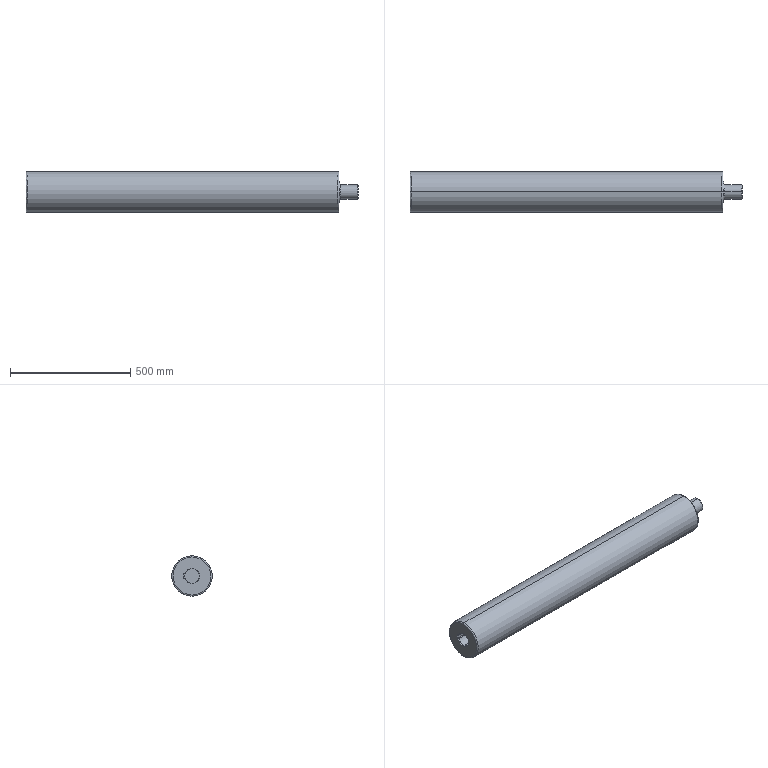Part | SolidWorks | features BaseBody 1 | 1 solid | 37 faces | box 1379 x 168 x 168 mm | volume 11660432 mm3 | cylinder 13 | plane 11 | spline 8 | cone 5 | commonest cylinder face diameters 60 x7 72 x2 146 x2 168 x2